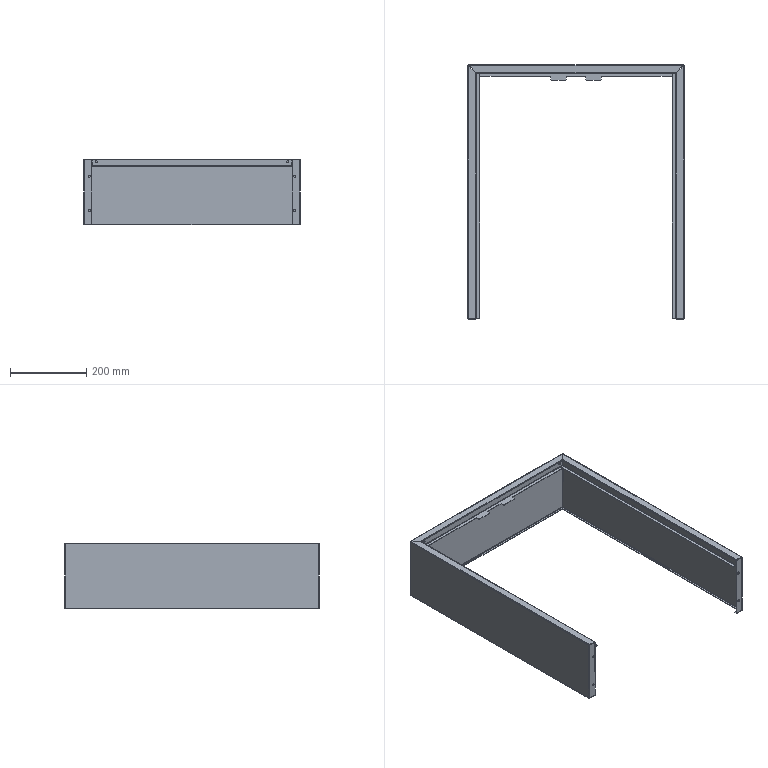Part | SolidWorks | features EdgeFlange 5, ICE 3, Fillet 2, SMBaseFlange 2, Cut 1, FlatPattern 1, MirrorPattern 1, SheetMetal 1 | 1 solid | 176 faces | box 568.4 x 668.4 x 173.4 mm | volume 516143 mm3 | plane 108 | cylinder 52 | spline 16 | commonest cylinder face diameters 1 x18 3.4 x18 6 x16